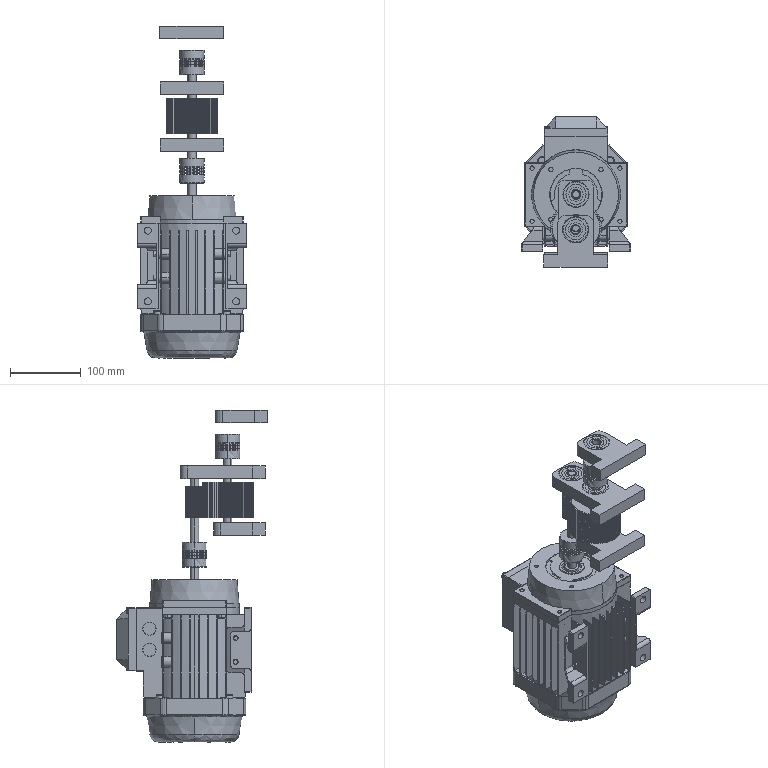Part | SolidWorks | features AEMSimFeature 1 | 19 solids | 2648 faces | box 154 x 213.028 x 468.972 mm | volume 4044827 mm3 | plane 1404 | cylinder 840 | spline 340 | cone 48 | torus 16 | commonest cylinder face diameters 0.5 x230 67.5 x71 72 x70 12 x38 20 x38 10 x34